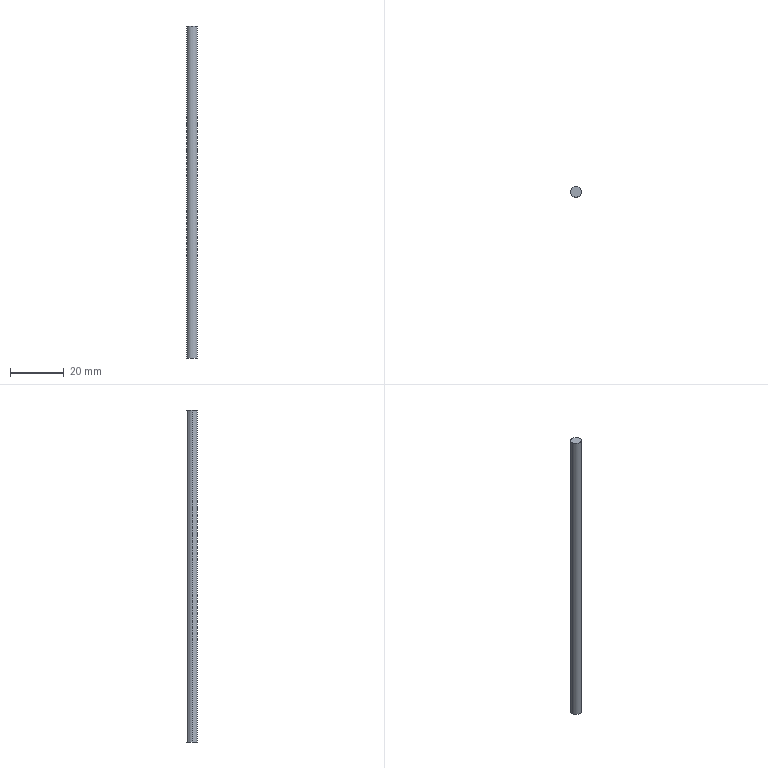Part | SolidWorks | features Extrusion 1 | 1 solid | 4 faces | box 4 x 4 x 124 mm | volume 1558 mm3 | cylinder 2 | plane 2 | commonest cylinder face diameters 4 x2
STEP:
#1=CARTESIAN_POINT('',(2.,0.,62.));
#2=VERTEX_POINT('',#1);
#3=CARTESIAN_POINT('',(-2.,0.,62.));
#4=VERTEX_POINT('',#3);
#5=CARTESIAN_POINT('',(0.,0.,62.));
#6=DIRECTION('',(0.,0.,1.));
#7=DIRECTION('',(1.,0.,0.));
#8=AXIS2_PLACEMENT_3D('',#5,#6,#7);
#9=CIRCLE('',#8,2.);
#10=EDGE_CURVE('',#2,#4,#9,.T.);
#11=ORIENTED_EDGE('',*,*,#10,.F.);
#12=CARTESIAN_POINT('',(2.,0.,-62.));
#13=VERTEX_POINT('',#12);
#14=CARTESIAN_POINT('',(2.,0.,62.));
#15=DIRECTION('',(0.,0.,-1.));
#16=VECTOR('',#15,1000.);
#17=LINE('',#14,#16);
#18=EDGE_CURVE('',#2,#13,#17,.T.);
#19=ORIENTED_EDGE('',*,*,#18,.T.);
#20=CARTESIAN_POINT('',(-2.,0.,-62.));
#21=VERTEX_POINT('',#20);
#22=CARTESIAN_POINT('',(0.,0.,-62.));
#23=DIRECTION('',(0.,0.,1.));
#24=DIRECTION('',(1.,0.,0.));
#25=AXIS2_PLACEMENT_3D('',#22,#23,#24);
#26=CIRCLE('',#25,2.);
#27=EDGE_CURVE('',#13,#21,#26,.T.);
#28=ORIENTED_EDGE('',*,*,#27,.T.);
#29=CARTESIAN_POINT('',(-2.,0.,62.));
#30=DIRECTION('',(0.,0.,-1.));
#31=VECTOR('',#30,1000.);
#32=LINE('',#29,#31);
#33=EDGE_CURVE('',#4,#21,#32,.T.);
#34=ORIENTED_EDGE('',*,*,#33,.F.);
#35=EDGE_LOOP('',(#11,#19,#28,#34));
#36=FACE_OUTER_BOUND('',#35,.T.);
#37=CARTESIAN_POINT('',(0.,0.,62.));
#38=DIRECTION('',(0.,0.,-1.));
#39=DIRECTION('',(-1.,0.,0.));
#40=AXIS2_PLACEMENT_3D('',#37,#38,#39);
#41=CYLINDRICAL_SURFACE('',#40,2.);
#42=ADVANCED_FACE('',(#36),#41,.T.);
#43=ORIENTED_EDGE('',*,*,#18,.F.);
#44=CARTESIAN_POINT('',(0.,0.,62.));
#45=DIRECTION('',(0.,0.,1.));
#46=DIRECTION('',(1.,0.,0.));
#47=AXIS2_PLACEMENT_3D('',#44,#45,#46);
#48=CIRCLE('',#47,2.);
#49=EDGE_CURVE('',#4,#2,#48,.T.);
#50=ORIENTED_EDGE('',*,*,#49,.F.);
#51=ORIENTED_EDGE('',*,*,#33,.T.);
#52=CARTESIAN_POINT('',(0.,0.,-62.));
#53=DIRECTION('',(0.,0.,1.));
#54=DIRECTION('',(1.,0.,0.));
#55=AXIS2_PLACEMENT_3D('',#52,#53,#54);
#56=CIRCLE('',#55,2.);
#57=EDGE_CURVE('',#21,#13,#56,.T.);
#58=ORIENTED_EDGE('',*,*,#57,.T.);
#59=EDGE_LOOP('',(#43,#50,#51,#58));
#60=FACE_OUTER_BOUND('',#59,.T.);
#61=CARTESIAN_POINT('',(0.,0.,62.));
#62=DIRECTION('',(0.,0.,-1.));
#63=DIRECTION('',(-1.,0.,0.));
#64=AXIS2_PLACEMENT_3D('',#61,#62,#63);
#65=CYLINDRICAL_SURFACE('',#64,2.);
#66=ADVANCED_FACE('',(#60),#65,.T.);
#67=ORIENTED_EDGE('',*,*,#49,.T.);
#68=ORIENTED_EDGE('',*,*,#10,.T.);
#69=EDGE_LOOP('',(#67,#68));
#70=FACE_OUTER_BOUND('',#69,.T.);
#71=CARTESIAN_POINT('',(0.,0.,62.));
#72=DIRECTION('',(0.,0.,1.));
#73=DIRECTION('',(1.,0.,0.));
#74=AXIS2_PLACEMENT_3D('',#71,#72,#73);
#75=PLANE('',#74);
#76=ADVANCED_FACE('',(#70),#75,.T.);
#77=ORIENTED_EDGE('',*,*,#57,.F.);
#78=ORIENTED_EDGE('',*,*,#27,.F.);
#79=EDGE_LOOP('',(#77,#78));
#80=FACE_OUTER_BOUND('',#79,.T.);
#81=CARTESIAN_POINT('',(0.,0.,-62.));
#82=DIRECTION('',(0.,0.,1.));
#83=DIRECTION('',(1.,0.,0.));
#84=AXIS2_PLACEMENT_3D('',#81,#82,#83);
#85=PLANE('',#84);
#86=ADVANCED_FACE('',(#80),#85,.F.);
#87=CLOSED_SHELL('',(#42,#66,#76,#86));
#88=MANIFOLD_SOLID_BREP('',#87);
#89=CARTESIAN_POINT('',(0.,0.,0.));
#90=DIRECTION('',(0.,0.,1.));
#91=DIRECTION('',(1.,0.,0.));
#92=AXIS2_PLACEMENT_3D('',#89,#90,#91);
#93=(LENGTH_UNIT()NAMED_UNIT(*)SI_UNIT(.MILLI.,.METRE.));
#94=UNCERTAINTY_MEASURE_WITH_UNIT(LENGTH_MEASURE(0.00001),#93,'','');
#95=(NAMED_UNIT(*)PLANE_ANGLE_UNIT()SI_UNIT($,.RADIAN.));
#96=(NAMED_UNIT(*)SI_UNIT($,.STERADIAN.)SOLID_ANGLE_UNIT());
#97=(GEOMETRIC_REPRESENTATION_CONTEXT(3)GLOBAL_UNCERTAINTY_ASSIGNED_CONTEXT((#94))GLOBAL_UNIT_ASSIGNED_CONTEXT((#93,#95,#96))REPRESENTATION_CONTEXT('',''));
#98=ADVANCED_BREP_SHAPE_REPRESENTATION('',(#88,#92),#97);